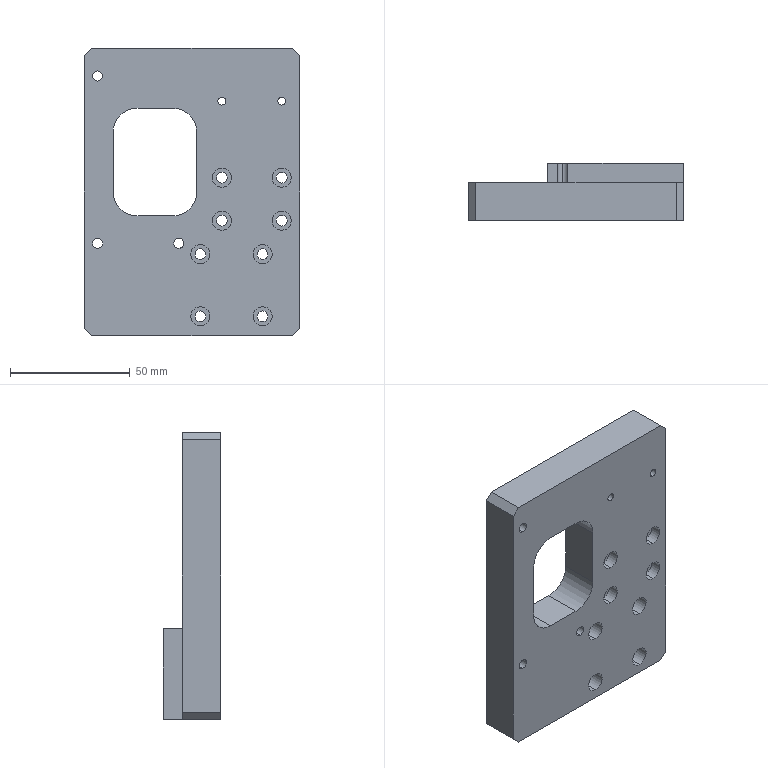Part | STEP file | slide fixing plate | 1 solid | 72 faces | box 90 x 24 x 120 mm | volume 159761 mm3 | cylinder 46 | plane 26 | commonest cylinder face diameters 4.5 x16 8 x16 4.2 x6 3.3 x4 20 x4